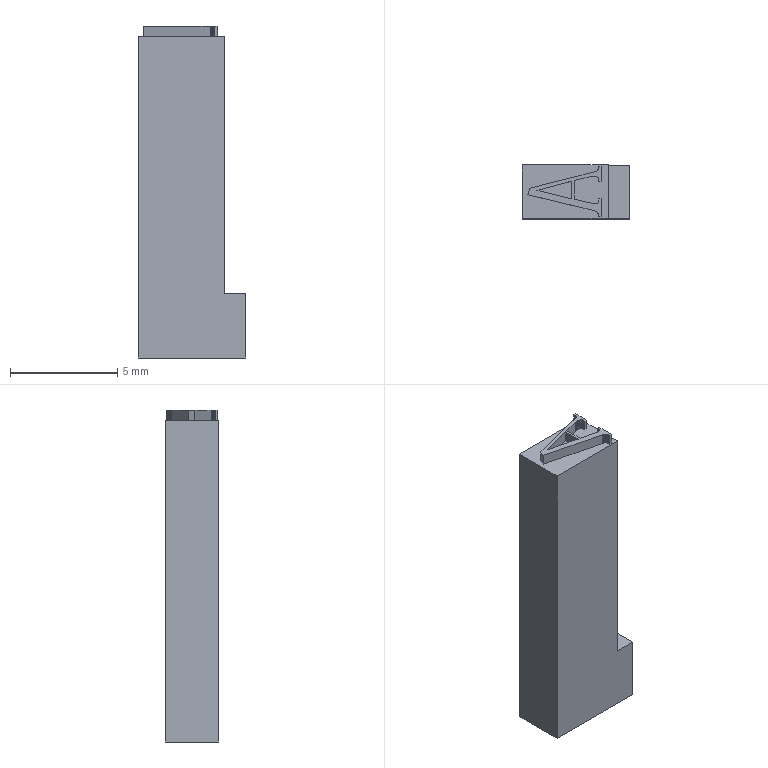Part | NX | features DIE-24 2 | 1 solid | 74 faces | box 5 x 2.5 x 15.5 mm | volume 158.423 mm3 | plane 74